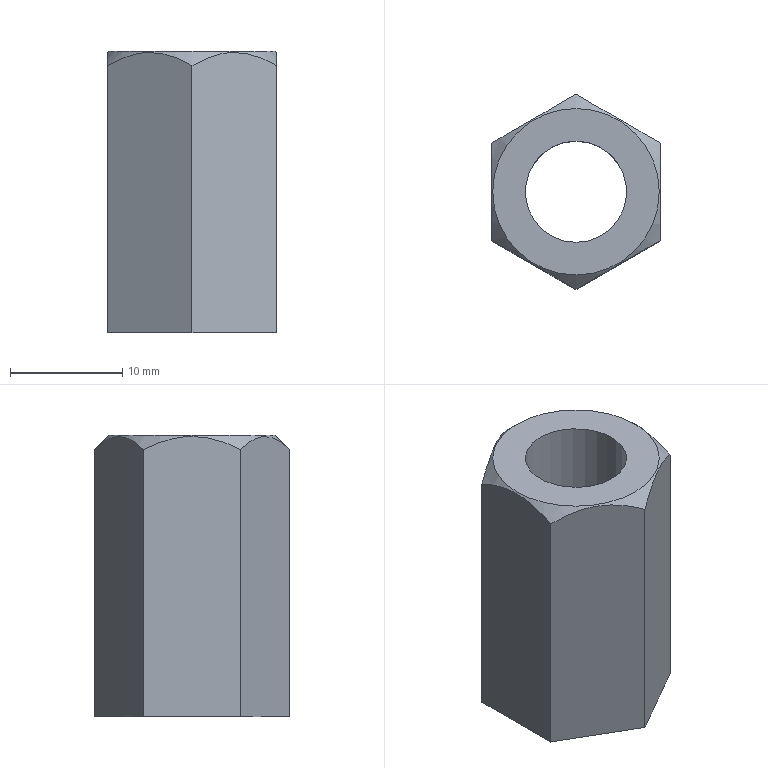Part | STEP file | 1 solid | 16 faces | box 15 x 17.321 x 25 mm | volume 2729 mm3 | plane 10 | cone 3 | cylinder 3 | commonest cylinder face diameters 9 x1 10.917 x1 12.5 x1
STEP:
#1=CARTESIAN_POINT('',(0.,0.,0.));
#2=DIRECTION('',(0.,0.,1.));
#3=DIRECTION('',(1.,0.,0.));
#4=AXIS2_PLACEMENT_3D('',#1,#2,#3);
#5=CARTESIAN_POINT('',(0.,-7.4,25.));
#6=VERTEX_POINT('',#5);
#7=CARTESIAN_POINT('',(0.,0.,25.));
#8=DIRECTION('',(0.,0.,-1.));
#9=DIRECTION('',(1.,0.,0.));
#10=AXIS2_PLACEMENT_3D('',#7,#8,#9);
#11=CIRCLE('',#10,7.4);
#12=CARTESIAN_POINT('',(0.,0.,23.4));
#13=DIRECTION('',(0.,0.,-1.));
#14=DIRECTION('',(0.,-1.,0.));
#15=AXIS2_PLACEMENT_3D('',#12,#13,#14);
#16=CONICAL_SURFACE('',#15,9.,0.7854);
#17=CARTESIAN_POINT('',(-1.571,-1.6));
#18=DIRECTION('',(1.,0.));
#19=VECTOR('',#18,1.);
#20=LINE('',#17,#19);
#21=(GEOMETRIC_REPRESENTATION_CONTEXT(2)PARAMETRIC_REPRESENTATION_CONTEXT()REPRESENTATION_CONTEXT('',''));
#22=DEFINITIONAL_REPRESENTATION('',(#20),#21);
#23=PCURVE('',#16,#22);
#24=CARTESIAN_POINT('',(0.,3.7,25.));
#25=DIRECTION('',(0.,0.,-1.));
#26=DIRECTION('',(-1.,0.,0.));
#27=AXIS2_PLACEMENT_3D('',#24,#25,#26);
#28=PLANE('',#27);
#29=CARTESIAN_POINT('',(0.,-3.7));
#30=DIRECTION('',(-1.,0.));
#31=AXIS2_PLACEMENT_2D('',#29,#30);
#32=CIRCLE('',#31,7.4);
#33=(GEOMETRIC_REPRESENTATION_CONTEXT(2)PARAMETRIC_REPRESENTATION_CONTEXT()REPRESENTATION_CONTEXT('',''));
#34=DEFINITIONAL_REPRESENTATION('',(#32),#33);
#35=PCURVE('',#28,#34);
#36=SURFACE_CURVE('',#11,(#23,#35),.PCURVE_S1.);
#37=EDGE_CURVE('',#6,#6,#36,.T.);
#38=ORIENTED_EDGE('',*,*,#37,.T.);
#39=CARTESIAN_POINT('',(0.,-8.66,23.74));
#40=VERTEX_POINT('',#39);
#41=CARTESIAN_POINT('',(0.,-7.4,25.));
#42=CARTESIAN_POINT('',(0.,-8.66,23.74));
#43=B_SPLINE_CURVE_WITH_KNOTS('',1,(#41,#42),.UNSPECIFIED.,.F.,.F.,(2,2),(-2.263,-0.4805),.PIECEWISE_BEZIER_KNOTS.);
#44=CARTESIAN_POINT('',(6.283,0.));
#45=DIRECTION('',(0.,1.));
#46=VECTOR('',#45,1.);
#47=LINE('',#44,#46);
#48=(GEOMETRIC_REPRESENTATION_CONTEXT(2)PARAMETRIC_REPRESENTATION_CONTEXT()REPRESENTATION_CONTEXT('',''));
#49=DEFINITIONAL_REPRESENTATION('',(#47),#48);
#50=PCURVE('',#16,#49);
#51=CARTESIAN_POINT('',(0.,0.));
#52=DIRECTION('',(0.,1.));
#53=VECTOR('',#52,1.);
#54=LINE('',#51,#53);
#55=(GEOMETRIC_REPRESENTATION_CONTEXT(2)PARAMETRIC_REPRESENTATION_CONTEXT()REPRESENTATION_CONTEXT('',''));
#56=DEFINITIONAL_REPRESENTATION('',(#54),#55);
#57=PCURVE('',#16,#56);
#58=SEAM_CURVE('',#43,(#50,#57),.PCURVE_S1.);
#59=EDGE_CURVE('',#6,#40,#58,.T.);
#60=ORIENTED_EDGE('',*,*,#59,.T.);
#61=CARTESIAN_POINT('',(7.5,-4.33,23.74));
#62=VERTEX_POINT('',#61);
#63=CARTESIAN_POINT('',(31.937,9.778,-1.));
#64=CARTESIAN_POINT('',(3.75,-6.495,30.716));
#65=CARTESIAN_POINT('',(-24.437,-22.769,-1.));
#66=(BOUNDED_CURVE()B_SPLINE_CURVE(2,(#63,#64,#65),.UNSPECIFIED.,.F.,.F.)B_SPLINE_CURVE_WITH_KNOTS((3,3),(0.,8.319),.PIECEWISE_BEZIER_KNOTS.)CURVE()GEOMETRIC_REPRESENTATION_ITEM()RATIONAL_B_SPLINE_CURVE((1.,4.453,1.))REPRESENTATION_ITEM(''));
#67=CARTESIAN_POINT('',(5.236,-0.3397));
#68=CARTESIAN_POINT('',(5.251,-0.4155));
#69=CARTESIAN_POINT('',(5.282,-0.558));
#70=CARTESIAN_POINT('',(5.328,-0.7466));
#71=CARTESIAN_POINT('',(5.375,-0.9116));
#72=CARTESIAN_POINT('',(5.422,-1.054));
#73=CARTESIAN_POINT('',(5.469,-1.176));
#74=CARTESIAN_POINT('',(5.517,-1.277));
#75=CARTESIAN_POINT('',(5.565,-1.359));
#76=CARTESIAN_POINT('',(5.614,-1.423));
#77=CARTESIAN_POINT('',(5.662,-1.467));
#78=CARTESIAN_POINT('',(5.711,-1.494));
#79=CARTESIAN_POINT('',(5.76,-1.503));
#80=CARTESIAN_POINT('',(5.808,-1.494));
#81=CARTESIAN_POINT('',(5.857,-1.467));
#82=CARTESIAN_POINT('',(5.906,-1.423));
#83=CARTESIAN_POINT('',(5.954,-1.359));
#84=CARTESIAN_POINT('',(6.002,-1.277));
#85=CARTESIAN_POINT('',(6.05,-1.176));
#86=CARTESIAN_POINT('',(6.097,-1.054));
#87=CARTESIAN_POINT('',(6.145,-0.9116));
#88=CARTESIAN_POINT('',(6.191,-0.7466));
#89=CARTESIAN_POINT('',(6.238,-0.558));
#90=CARTESIAN_POINT('',(6.268,-0.4155));
#91=CARTESIAN_POINT('',(6.283,-0.3397));
#92=B_SPLINE_CURVE_WITH_KNOTS('',3,(#67,#68,#69,#70,#71,#72,#73,#74,#75,#76,#77,#78,#79,#80,#81,#82,#83,#84,#85,#86,#87,#88,#89,#90,#91),.UNSPECIFIED.,.F.,.F.,(4,1,1,1,1,1,1,1,1,1,1,1,1,1,1,1,1,1,1,1,1,1,4),(2.759,2.886,3.014,3.141,3.268,3.396,3.523,3.65,3.777,3.905,4.032,4.159,4.287,4.414,4.541,4.669,4.796,4.923,5.051,5.178,5.305,5.433,5.56),.QUASI_UNIFORM_KNOTS.);
#93=(GEOMETRIC_REPRESENTATION_CONTEXT(2)PARAMETRIC_REPRESENTATION_CONTEXT()REPRESENTATION_CONTEXT('',''));
#94=DEFINITIONAL_REPRESENTATION('',(#92),#93);
#95=PCURVE('',#16,#94);
#96=CARTESIAN_POINT('',(-7.5,-12.99,0.));
#97=DIRECTION('',(-0.5,0.866,0.));
#98=DIRECTION('',(0.,0.,1.));
#99=AXIS2_PLACEMENT_3D('',#96,#97,#98);
#100=PLANE('',#99);
#101=CARTESIAN_POINT('',(-1.,45.537));
#102=CARTESIAN_POINT('',(30.716,12.99));
#103=CARTESIAN_POINT('',(-1.,-19.557));
#104=(BOUNDED_CURVE()B_SPLINE_CURVE(2,(#101,#102,#103),.UNSPECIFIED.,.F.,.F.)B_SPLINE_CURVE_WITH_KNOTS((3,3),(0.,8.319),.PIECEWISE_BEZIER_KNOTS.)CURVE()GEOMETRIC_REPRESENTATION_ITEM()RATIONAL_B_SPLINE_CURVE((1.,4.453,1.))REPRESENTATION_ITEM(''));
#105=(GEOMETRIC_REPRESENTATION_CONTEXT(2)PARAMETRIC_REPRESENTATION_CONTEXT()REPRESENTATION_CONTEXT('',''));
#106=DEFINITIONAL_REPRESENTATION('',(#104),#105);
#107=PCURVE('',#100,#106);
#108=SURFACE_CURVE('',#66,(#95,#107),.PCURVE_S1.);
#109=EDGE_CURVE('',#62,#40,#108,.T.);
#110=ORIENTED_EDGE('',*,*,#109,.F.);
#111=CARTESIAN_POINT('',(7.5,4.33,23.74));
#112=VERTEX_POINT('',#111);
#113=CARTESIAN_POINT('',(7.5,32.547,-1.));
#114=CARTESIAN_POINT('',(7.5,0.,30.716));
#115=CARTESIAN_POINT('',(7.5,-32.547,-1.));
#116=(BOUNDED_CURVE()B_SPLINE_CURVE(2,(#113,#114,#115),.UNSPECIFIED.,.F.,.F.)B_SPLINE_CURVE_WITH_KNOTS((3,3),(0.,8.319),.PIECEWISE_BEZIER_KNOTS.)CURVE()GEOMETRIC_REPRESENTATION_ITEM()RATIONAL_B_SPLINE_CURVE((1.,4.453,1.))REPRESENTATION_ITEM(''));
#117=CARTESIAN_POINT('',(4.189,-0.3397));
#118=CARTESIAN_POINT('',(4.204,-0.4155));
#119=CARTESIAN_POINT('',(4.234,-0.558));
#120=CARTESIAN_POINT('',(4.281,-0.7466));
#121=CARTESIAN_POINT('',(4.327,-0.9116));
#122=CARTESIAN_POINT('',(4.375,-1.054));
#123=CARTESIAN_POINT('',(4.422,-1.176));
#124=CARTESIAN_POINT('',(4.47,-1.277));
#125=CARTESIAN_POINT('',(4.518,-1.359));
#126=CARTESIAN_POINT('',(4.566,-1.423));
#127=CARTESIAN_POINT('',(4.615,-1.467));
#128=CARTESIAN_POINT('',(4.664,-1.494));
#129=CARTESIAN_POINT('',(4.712,-1.503));
#130=CARTESIAN_POINT('',(4.761,-1.494));
#131=CARTESIAN_POINT('',(4.81,-1.467));
#132=CARTESIAN_POINT('',(4.858,-1.423));
#133=CARTESIAN_POINT('',(4.907,-1.359));
#134=CARTESIAN_POINT('',(4.955,-1.277));
#135=CARTESIAN_POINT('',(5.003,-1.176));
#136=CARTESIAN_POINT('',(5.05,-1.054));
#137=CARTESIAN_POINT('',(5.097,-0.9116));
#138=CARTESIAN_POINT('',(5.144,-0.7466));
#139=CARTESIAN_POINT('',(5.19,-0.558));
#140=CARTESIAN_POINT('',(5.221,-0.4155));
#141=CARTESIAN_POINT('',(5.236,-0.3397));
#142=B_SPLINE_CURVE_WITH_KNOTS('',3,(#117,#118,#119,#120,#121,#122,#123,#124,#125,#126,#127,#128,#129,#130,#131,#132,#133,#134,#135,#136,#137,#138,#139,#140,#141),.UNSPECIFIED.,.F.,.F.,(4,1,1,1,1,1,1,1,1,1,1,1,1,1,1,1,1,1,1,1,1,1,4),(2.759,2.886,3.014,3.141,3.268,3.396,3.523,3.65,3.777,3.905,4.032,4.159,4.287,4.414,4.541,4.669,4.796,4.923,5.051,5.178,5.305,5.433,5.56),.QUASI_UNIFORM_KNOTS.);
#143=(GEOMETRIC_REPRESENTATION_CONTEXT(2)PARAMETRIC_REPRESENTATION_CONTEXT()REPRESENTATION_CONTEXT('',''));
#144=DEFINITIONAL_REPRESENTATION('',(#142),#143);
#145=PCURVE('',#16,#144);
#146=CARTESIAN_POINT('',(7.5,-4.33,0.));
#147=DIRECTION('',(-1.,0.,0.));
#148=DIRECTION('',(0.,0.,1.));
#149=AXIS2_PLACEMENT_3D('',#146,#147,#148);
#150=PLANE('',#149);
#151=CARTESIAN_POINT('',(-1.,36.877));
#152=CARTESIAN_POINT('',(30.716,4.33));
#153=CARTESIAN_POINT('',(-1.,-28.217));
#154=(BOUNDED_CURVE()B_SPLINE_CURVE(2,(#151,#152,#153),.UNSPECIFIED.,.F.,.F.)B_SPLINE_CURVE_WITH_KNOTS((3,3),(0.,8.319),.PIECEWISE_BEZIER_KNOTS.)CURVE()GEOMETRIC_REPRESENTATION_ITEM()RATIONAL_B_SPLINE_CURVE((1.,4.453,1.))REPRESENTATION_ITEM(''));
#155=(GEOMETRIC_REPRESENTATION_CONTEXT(2)PARAMETRIC_REPRESENTATION_CONTEXT()REPRESENTATION_CONTEXT('',''));
#156=DEFINITIONAL_REPRESENTATION('',(#154),#155);
#157=PCURVE('',#150,#156);
#158=SURFACE_CURVE('',#116,(#145,#157),.PCURVE_S1.);
#159=EDGE_CURVE('',#112,#62,#158,.T.);
#160=ORIENTED_EDGE('',*,*,#159,.F.);
#161=CARTESIAN_POINT('',(0.,8.66,23.74));
#162=VERTEX_POINT('',#161);
#163=CARTESIAN_POINT('',(-24.437,22.769,-1.));
#164=CARTESIAN_POINT('',(3.75,6.495,30.716));
#165=CARTESIAN_POINT('',(31.937,-9.778,-1.));
#166=(BOUNDED_CURVE()B_SPLINE_CURVE(2,(#163,#164,#165),.UNSPECIFIED.,.F.,.F.)B_SPLINE_CURVE_WITH_KNOTS((3,3),(0.,8.319),.PIECEWISE_BEZIER_KNOTS.)CURVE()GEOMETRIC_REPRESENTATION_ITEM()RATIONAL_B_SPLINE_CURVE((1.,4.453,1.))REPRESENTATION_ITEM(''));
#167=CARTESIAN_POINT('',(3.142,-0.3397));
#168=CARTESIAN_POINT('',(3.157,-0.4155));
#169=CARTESIAN_POINT('',(3.187,-0.558));
#170=CARTESIAN_POINT('',(3.233,-0.7466));
#171=CARTESIAN_POINT('',(3.28,-0.9116));
#172=CARTESIAN_POINT('',(3.327,-1.054));
#173=CARTESIAN_POINT('',(3.375,-1.176));
#174=CARTESIAN_POINT('',(3.423,-1.277));
#175=CARTESIAN_POINT('',(3.471,-1.359));
#176=CARTESIAN_POINT('',(3.519,-1.423));
#177=CARTESIAN_POINT('',(3.568,-1.467));
#178=CARTESIAN_POINT('',(3.616,-1.494));
#179=CARTESIAN_POINT('',(3.665,-1.503));
#180=CARTESIAN_POINT('',(3.714,-1.494));
#181=CARTESIAN_POINT('',(3.763,-1.467));
#182=CARTESIAN_POINT('',(3.811,-1.423));
#183=CARTESIAN_POINT('',(3.859,-1.359));
#184=CARTESIAN_POINT('',(3.908,-1.277));
#185=CARTESIAN_POINT('',(3.956,-1.176));
#186=CARTESIAN_POINT('',(4.003,-1.054));
#187=CARTESIAN_POINT('',(4.05,-0.9116));
#188=CARTESIAN_POINT('',(4.097,-0.7466));
#189=CARTESIAN_POINT('',(4.143,-0.558));
#190=CARTESIAN_POINT('',(4.174,-0.4155));
#191=CARTESIAN_POINT('',(4.189,-0.3397));
#192=B_SPLINE_CURVE_WITH_KNOTS('',3,(#167,#168,#169,#170,#171,#172,#173,#174,#175,#176,#177,#178,#179,#180,#181,#182,#183,#184,#185,#186,#187,#188,#189,#190,#191),.UNSPECIFIED.,.F.,.F.,(4,1,1,1,1,1,1,1,1,1,1,1,1,1,1,1,1,1,1,1,1,1,4),(2.759,2.886,3.014,3.141,3.268,3.396,3.523,3.65,3.777,3.905,4.032,4.159,4.287,4.414,4.541,4.669,4.796,4.923,5.051,5.178,5.305,5.433,5.56),.QUASI_UNIFORM_KNOTS.);
#193=(GEOMETRIC_REPRESENTATION_CONTEXT(2)PARAMETRIC_REPRESENTATION_CONTEXT()REPRESENTATION_CONTEXT('',''));
#194=DEFINITIONAL_REPRESENTATION('',(#192),#193);
#195=PCURVE('',#16,#194);
#196=CARTESIAN_POINT('',(7.5,4.33,0.));
#197=DIRECTION('',(-0.5,-0.866,0.));
#198=DIRECTION('',(0.,0.,1.));
#199=AXIS2_PLACEMENT_3D('',#196,#197,#198);
#200=PLANE('',#199);
#201=CARTESIAN_POINT('',(-1.,36.877));
#202=CARTESIAN_POINT('',(30.716,4.33));
#203=CARTESIAN_POINT('',(-1.,-28.217));
#204=(BOUNDED_CURVE()B_SPLINE_CURVE(2,(#201,#202,#203),.UNSPECIFIED.,.F.,.F.)B_SPLINE_CURVE_WITH_KNOTS((3,3),(0.,8.319),.PIECEWISE_BEZIER_KNOTS.)CURVE()GEOMETRIC_REPRESENTATION_ITEM()RATIONAL_B_SPLINE_CURVE((1.,4.453,1.))REPRESENTATION_ITEM(''));
#205=(GEOMETRIC_REPRESENTATION_CONTEXT(2)PARAMETRIC_REPRESENTATION_CONTEXT()REPRESENTATION_CONTEXT('',''));
#206=DEFINITIONAL_REPRESENTATION('',(#204),#205);
#207=PCURVE('',#200,#206);
#208=SURFACE_CURVE('',#166,(#195,#207),.PCURVE_S1.);
#209=EDGE_CURVE('',#162,#112,#208,.T.);
#210=ORIENTED_EDGE('',*,*,#209,.F.);
#211=CARTESIAN_POINT('',(-7.5,4.33,23.74));
#212=VERTEX_POINT('',#211);
#213=CARTESIAN_POINT('',(-31.937,-9.778,-1.));
#214=CARTESIAN_POINT('',(-3.75,6.495,30.716));
#215=CARTESIAN_POINT('',(24.437,22.769,-1.));
#216=(BOUNDED_CURVE()B_SPLINE_CURVE(2,(#213,#214,#215),.UNSPECIFIED.,.F.,.F.)B_SPLINE_CURVE_WITH_KNOTS((3,3),(0.,8.319),.PIECEWISE_BEZIER_KNOTS.)CURVE()GEOMETRIC_REPRESENTATION_ITEM()RATIONAL_B_SPLINE_CURVE((1.,4.453,1.))REPRESENTATION_ITEM(''));
#217=CARTESIAN_POINT('',(2.094,-0.3397));
#218=CARTESIAN_POINT('',(2.11,-0.4155));
#219=CARTESIAN_POINT('',(2.14,-0.558));
#220=CARTESIAN_POINT('',(2.186,-0.7466));
#221=CARTESIAN_POINT('',(2.233,-0.9116));
#222=CARTESIAN_POINT('',(2.28,-1.054));
#223=CARTESIAN_POINT('',(2.328,-1.176));
#224=CARTESIAN_POINT('',(2.376,-1.277));
#225=CARTESIAN_POINT('',(2.424,-1.359));
#226=CARTESIAN_POINT('',(2.472,-1.423));
#227=CARTESIAN_POINT('',(2.521,-1.467));
#228=CARTESIAN_POINT('',(2.569,-1.494));
#229=CARTESIAN_POINT('',(2.618,-1.503));
#230=CARTESIAN_POINT('',(2.667,-1.494));
#231=CARTESIAN_POINT('',(2.715,-1.467));
#232=CARTESIAN_POINT('',(2.764,-1.423));
#233=CARTESIAN_POINT('',(2.812,-1.359));
#234=CARTESIAN_POINT('',(2.86,-1.277));
#235=CARTESIAN_POINT('',(2.908,-1.176));
#236=CARTESIAN_POINT('',(2.956,-1.054));
#237=CARTESIAN_POINT('',(3.003,-0.9116));
#238=CARTESIAN_POINT('',(3.05,-0.7466));
#239=CARTESIAN_POINT('',(3.096,-0.558));
#240=CARTESIAN_POINT('',(3.126,-0.4155));
#241=CARTESIAN_POINT('',(3.142,-0.3397));
#242=B_SPLINE_CURVE_WITH_KNOTS('',3,(#217,#218,#219,#220,#221,#222,#223,#224,#225,#226,#227,#228,#229,#230,#231,#232,#233,#234,#235,#236,#237,#238,#239,#240,#241),.UNSPECIFIED.,.F.,.F.,(4,1,1,1,1,1,1,1,1,1,1,1,1,1,1,1,1,1,1,1,1,1,4),(2.759,2.886,3.014,3.141,3.268,3.396,3.523,3.65,3.777,3.905,4.032,4.159,4.287,4.414,4.541,4.669,4.796,4.923,5.051,5.178,5.305,5.433,5.56),.QUASI_UNIFORM_KNOTS.);
#243=(GEOMETRIC_REPRESENTATION_CONTEXT(2)PARAMETRIC_REPRESENTATION_CONTEXT()REPRESENTATION_CONTEXT('',''));
#244=DEFINITIONAL_REPRESENTATION('',(#242),#243);
#245=PCURVE('',#16,#244);
#246=CARTESIAN_POINT('',(7.5,12.99,0.));
#247=DIRECTION('',(0.5,-0.866,0.));
#248=DIRECTION('',(0.,0.,-1.));
#249=AXIS2_PLACEMENT_3D('',#246,#247,#248);
#250=PLANE('',#249);
#251=CARTESIAN_POINT('',(1.,-45.537));
#252=CARTESIAN_POINT('',(-30.716,-12.99));
#253=CARTESIAN_POINT('',(1.,19.557));
#254=(BOUNDED_CURVE()B_SPLINE_CURVE(2,(#251,#252,#253),.UNSPECIFIED.,.F.,.F.)B_SPLINE_CURVE_WITH_KNOTS((3,3),(0.,8.319),.PIECEWISE_BEZIER_KNOTS.)CURVE()GEOMETRIC_REPRESENTATION_ITEM()RATIONAL_B_SPLINE_CURVE((1.,4.453,1.))REPRESENTATION_ITEM(''));
#255=(GEOMETRIC_REPRESENTATION_CONTEXT(2)PARAMETRIC_REPRESENTATION_CONTEXT()REPRESENTATION_CONTEXT('',''));
#256=DEFINITIONAL_REPRESENTATION('',(#254),#255);
#257=PCURVE('',#250,#256);
#258=SURFACE_CURVE('',#216,(#245,#257),.PCURVE_S1.);
#259=EDGE_CURVE('',#212,#162,#258,.T.);
#260=ORIENTED_EDGE('',*,*,#259,.F.);
#261=CARTESIAN_POINT('',(-7.5,-4.33,23.74));
#262=VERTEX_POINT('',#261);
#263=CARTESIAN_POINT('',(-7.5,-32.547,-1.));
#264=CARTESIAN_POINT('',(-7.5,0.,30.716));
#265=CARTESIAN_POINT('',(-7.5,32.547,-1.));
#266=(BOUNDED_CURVE()B_SPLINE_CURVE(2,(#263,#264,#265),.UNSPECIFIED.,.F.,.F.)B_SPLINE_CURVE_WITH_KNOTS((3,3),(0.,8.319),.PIECEWISE_BEZIER_KNOTS.)CURVE()GEOMETRIC_REPRESENTATION_ITEM()RATIONAL_B_SPLINE_CURVE((1.,4.453,1.))REPRESENTATION_ITEM(''));
#267=CARTESIAN_POINT('',(1.047,-0.3397));
#268=CARTESIAN_POINT('',(1.062,-0.4155));
#269=CARTESIAN_POINT('',(1.093,-0.558));
#270=CARTESIAN_POINT('',(1.139,-0.7466));
#271=CARTESIAN_POINT('',(1.186,-0.9116));
#272=CARTESIAN_POINT('',(1.233,-1.054));
#273=CARTESIAN_POINT('',(1.28,-1.176));
#274=CARTESIAN_POINT('',(1.328,-1.277));
#275=CARTESIAN_POINT('',(1.376,-1.359));
#276=CARTESIAN_POINT('',(1.425,-1.423));
#277=CARTESIAN_POINT('',(1.473,-1.467));
#278=CARTESIAN_POINT('',(1.522,-1.494));
#279=CARTESIAN_POINT('',(1.571,-1.503));
#280=CARTESIAN_POINT('',(1.62,-1.494));
#281=CARTESIAN_POINT('',(1.668,-1.467));
#282=CARTESIAN_POINT('',(1.717,-1.423));
#283=CARTESIAN_POINT('',(1.765,-1.359));
#284=CARTESIAN_POINT('',(1.813,-1.277));
#285=CARTESIAN_POINT('',(1.861,-1.176));
#286=CARTESIAN_POINT('',(1.909,-1.054));
#287=CARTESIAN_POINT('',(1.956,-0.9116));
#288=CARTESIAN_POINT('',(2.003,-0.7466));
#289=CARTESIAN_POINT('',(2.049,-0.558));
#290=CARTESIAN_POINT('',(2.079,-0.4155));
#291=CARTESIAN_POINT('',(2.094,-0.3397));
#292=B_SPLINE_CURVE_WITH_KNOTS('',3,(#267,#268,#269,#270,#271,#272,#273,#274,#275,#276,#277,#278,#279,#280,#281,#282,#283,#284,#285,#286,#287,#288,#289,#290,#291),.UNSPECIFIED.,.F.,.F.,(4,1,1,1,1,1,1,1,1,1,1,1,1,1,1,1,1,1,1,1,1,1,4),(2.759,2.886,3.014,3.141,3.268,3.396,3.523,3.65,3.777,3.905,4.032,4.159,4.287,4.414,4.541,4.669,4.796,4.923,5.051,5.178,5.305,5.433,5.56),.QUASI_UNIFORM_KNOTS.);
#293=(GEOMETRIC_REPRESENTATION_CONTEXT(2)PARAMETRIC_REPRESENTATION_CONTEXT()REPRESENTATION_CONTEXT('',''));
#294=DEFINITIONAL_REPRESENTATION('',(#292),#293);
#295=PCURVE('',#16,#294);
#296=CARTESIAN_POINT('',(-7.5,4.33,0.));
#297=DIRECTION('',(1.,0.,0.));
#298=DIRECTION('',(0.,0.,-1.));
#299=AXIS2_PLACEMENT_3D('',#296,#297,#298);
#300=PLANE('',#299);
#301=CARTESIAN_POINT('',(1.,-36.877));
#302=CARTESIAN_POINT('',(-30.716,-4.33));
#303=CARTESIAN_POINT('',(1.,28.217));
#304=(BOUNDED_CURVE()B_SPLINE_CURVE(2,(#301,#302,#303),.UNSPECIFIED.,.F.,.F.)B_SPLINE_CURVE_WITH_KNOTS((3,3),(0.,8.319),.PIECEWISE_BEZIER_KNOTS.)CURVE()GEOMETRIC_REPRESENTATION_ITEM()RATIONAL_B_SPLINE_CURVE((1.,4.453,1.))REPRESENTATION_ITEM(''));
#305=(GEOMETRIC_REPRESENTATION_CONTEXT(2)PARAMETRIC_REPRESENTATION_CONTEXT()REPRESENTATION_CONTEXT('',''));
#306=DEFINITIONAL_REPRESENTATION('',(#304),#305);
#307=PCURVE('',#300,#306);
#308=SURFACE_CURVE('',#266,(#295,#307),.PCURVE_S1.);
#309=EDGE_CURVE('',#262,#212,#308,.T.);
#310=ORIENTED_EDGE('',*,*,#309,.F.);
#311=CARTESIAN_POINT('',(24.437,-22.769,-1.));
#312=CARTESIAN_POINT('',(-3.75,-6.495,30.716));
#313=CARTESIAN_POINT('',(-31.937,9.778,-1.));
#314=(BOUNDED_CURVE()B_SPLINE_CURVE(2,(#311,#312,#313),.UNSPECIFIED.,.F.,.F.)B_SPLINE_CURVE_WITH_KNOTS((3,3),(0.,8.319),.PIECEWISE_BEZIER_KNOTS.)CURVE()GEOMETRIC_REPRESENTATION_ITEM()RATIONAL_B_SPLINE_CURVE((1.,4.453,1.))REPRESENTATION_ITEM(''));
#315=CARTESIAN_POINT('',(0.,-0.3397));
#316=CARTESIAN_POINT('',(0.01515,-0.4155));
#317=CARTESIAN_POINT('',(0.04564,-0.558));
#318=CARTESIAN_POINT('',(0.09189,-0.7466));
#319=CARTESIAN_POINT('',(0.1386,-0.9116));
#320=CARTESIAN_POINT('',(0.1858,-1.054));
#321=CARTESIAN_POINT('',(0.2333,-1.176));
#322=CARTESIAN_POINT('',(0.2812,-1.277));
#323=CARTESIAN_POINT('',(0.3293,-1.359));
#324=CARTESIAN_POINT('',(0.3777,-1.423));
#325=CARTESIAN_POINT('',(0.4262,-1.467));
#326=CARTESIAN_POINT('',(0.4749,-1.494));
#327=CARTESIAN_POINT('',(0.5236,-1.503));
#328=CARTESIAN_POINT('',(0.5723,-1.494));
#329=CARTESIAN_POINT('',(0.621,-1.467));
#330=CARTESIAN_POINT('',(0.6695,-1.423));
#331=CARTESIAN_POINT('',(0.7179,-1.359));
#332=CARTESIAN_POINT('',(0.766,-1.277));
#333=CARTESIAN_POINT('',(0.8139,-1.176));
#334=CARTESIAN_POINT('',(0.8614,-1.054));
#335=CARTESIAN_POINT('',(0.9086,-0.9116));
#336=CARTESIAN_POINT('',(0.9553,-0.7466));
#337=CARTESIAN_POINT('',(1.002,-0.558));
#338=CARTESIAN_POINT('',(1.032,-0.4155));
#339=CARTESIAN_POINT('',(1.047,-0.3397));
#340=B_SPLINE_CURVE_WITH_KNOTS('',3,(#315,#316,#317,#318,#319,#320,#321,#322,#323,#324,#325,#326,#327,#328,#329,#330,#331,#332,#333,#334,#335,#336,#337,#338,#339),.UNSPECIFIED.,.F.,.F.,(4,1,1,1,1,1,1,1,1,1,1,1,1,1,1,1,1,1,1,1,1,1,4),(2.759,2.886,3.014,3.141,3.268,3.396,3.523,3.65,3.777,3.905,4.032,4.159,4.287,4.414,4.541,4.669,4.796,4.923,5.051,5.178,5.305,5.433,5.56),.QUASI_UNIFORM_KNOTS.);
#341=(GEOMETRIC_REPRESENTATION_CONTEXT(2)PARAMETRIC_REPRESENTATION_CONTEXT()REPRESENTATION_CONTEXT('',''));
#342=DEFINITIONAL_REPRESENTATION('',(#340),#341);
#343=PCURVE('',#16,#342);
#344=CARTESIAN_POINT('',(-7.5,-4.33,0.));
#345=DIRECTION('',(0.5,0.866,0.));
#346=DIRECTION('',(0.,0.,-1.));
#347=AXIS2_PLACEMENT_3D('',#344,#345,#346);
#348=PLANE('',#347);
#349=CARTESIAN_POINT('',(1.,-36.877));
#350=CARTESIAN_POINT('',(-30.716,-4.33));
#351=CARTESIAN_POINT('',(1.,28.217));
#352=(BOUNDED_CURVE()B_SPLINE_CURVE(2,(#349,#350,#351),.UNSPECIFIED.,.F.,.F.)B_SPLINE_CURVE_WITH_KNOTS((3,3),(0.,8.319),.PIECEWISE_BEZIER_KNOTS.)CURVE()GEOMETRIC_REPRESENTATION_ITEM()RATIONAL_B_SPLINE_CURVE((1.,4.453,1.))REPRESENTATION_ITEM(''));
#353=(GEOMETRIC_REPRESENTATION_CONTEXT(2)PARAMETRIC_REPRESENTATION_CONTEXT()REPRESENTATION_CONTEXT('',''));
#354=DEFINITIONAL_REPRESENTATION('',(#352),#353);
#355=PCURVE('',#348,#354);
#356=SURFACE_CURVE('',#314,(#343,#355),.PCURVE_S1.);
#357=EDGE_CURVE('',#40,#262,#356,.T.);
#358=ORIENTED_EDGE('',*,*,#357,.F.);
#359=ORIENTED_EDGE('',*,*,#59,.F.);
#360=EDGE_LOOP('',(#38,#60,#110,#160,#210,#260,#310,#358,#359));
#361=FACE_BOUND('',#360,.T.);
#362=ADVANCED_FACE('',(#361),#16,.T.);
#363=ORIENTED_EDGE('',*,*,#37,.F.);
#364=EDGE_LOOP('',(#363));
#365=FACE_BOUND('',#364,.T.);
#366=CARTESIAN_POINT('',(0.,-4.5,25.));
#367=VERTEX_POINT('',#366);
#368=CARTESIAN_POINT('',(0.,0.,25.));
#369=DIRECTION('',(0.,0.,1.));
#370=DIRECTION('',(0.,1.,0.));
#371=AXIS2_PLACEMENT_3D('',#368,#369,#370);
#372=CIRCLE('',#371,4.5);
#373=CARTESIAN_POINT('',(0.,0.8));
#374=CARTESIAN_POINT('',(7.794,0.8));
#375=CARTESIAN_POINT('',(3.897,-5.95));
#376=CARTESIAN_POINT('',(0.,-12.7));
#377=CARTESIAN_POINT('',(-3.897,-5.95));
#378=CARTESIAN_POINT('',(-7.794,0.8));
#379=CARTESIAN_POINT('',(0.,0.8));
#380=(BOUNDED_CURVE()B_SPLINE_CURVE(2,(#373,#374,#375,#376,#377,#378,#379),.UNSPECIFIED.,.T.,.F.)B_SPLINE_CURVE_WITH_KNOTS((1,2,2,2,2,1),(-2.094,0.,2.094,4.189,6.283,8.378),.UNSPECIFIED.)CURVE()GEOMETRIC_REPRESENTATION_ITEM()RATIONAL_B_SPLINE_CURVE((1.,0.5,1.,0.5,1.,0.5,1.))REPRESENTATION_ITEM(''));
#381=(GEOMETRIC_REPRESENTATION_CONTEXT(2)PARAMETRIC_REPRESENTATION_CONTEXT()REPRESENTATION_CONTEXT('',''));
#382=DEFINITIONAL_REPRESENTATION('',(#380),#381);
#383=PCURVE('',#28,#382);
#384=CARTESIAN_POINT('',(0.,0.,20.25));
#385=DIRECTION('',(0.,0.,1.));
#386=DIRECTION('',(0.,-1.,0.));
#387=AXIS2_PLACEMENT_3D('',#384,#385,#386);
#388=CYLINDRICAL_SURFACE('',#387,4.5);
#389=CARTESIAN_POINT('',(-3.142,4.75));
#390=DIRECTION('',(1.,0.));
#391=VECTOR('',#390,1.);
#392=LINE('',#389,#391);
#393=(GEOMETRIC_REPRESENTATION_CONTEXT(2)PARAMETRIC_REPRESENTATION_CONTEXT()REPRESENTATION_CONTEXT('',''));
#394=DEFINITIONAL_REPRESENTATION('',(#392),#393);
#395=PCURVE('',#388,#394);
#396=SURFACE_CURVE('',#372,(#383,#395),.PCURVE_S1.);
#397=EDGE_CURVE('',#367,#367,#396,.T.);
#398=ORIENTED_EDGE('',*,*,#397,.F.);
#399=EDGE_LOOP('',(#398));
#400=FACE_BOUND('',#399,.T.);
#401=ADVANCED_FACE('',(#365,#400),#28,.F.);
#402=CARTESIAN_POINT('',(0.,8.66,0.));
#403=VERTEX_POINT('',#402);
#404=CARTESIAN_POINT('',(0.000000001,8.66,23.74));
#405=DIRECTION('',(0.,0.,-1.));
#406=VECTOR('',#405,1.);
#407=LINE('',#404,#406);
#408=CARTESIAN_POINT('',(-23.74,-8.66));
#409=DIRECTION('',(1.,0.));
#410=VECTOR('',#409,1.);
#411=LINE('',#408,#410);
#412=(GEOMETRIC_REPRESENTATION_CONTEXT(2)PARAMETRIC_REPRESENTATION_CONTEXT()REPRESENTATION_CONTEXT('',''));
#413=DEFINITIONAL_REPRESENTATION('',(#411),#412);
#414=PCURVE('',#250,#413);
#415=CARTESIAN_POINT('',(23.74,8.66));
#416=DIRECTION('',(-1.,0.));
#417=VECTOR('',#416,1.);
#418=LINE('',#415,#417);
#419=(GEOMETRIC_REPRESENTATION_CONTEXT(2)PARAMETRIC_REPRESENTATION_CONTEXT()REPRESENTATION_CONTEXT('',''));
#420=DEFINITIONAL_REPRESENTATION('',(#418),#419);
#421=PCURVE('',#200,#420);
#422=SURFACE_CURVE('',#407,(#414,#421),.PCURVE_S1.);
#423=EDGE_CURVE('',#162,#403,#422,.T.);
#424=ORIENTED_EDGE('',*,*,#423,.T.);
#425=CARTESIAN_POINT('',(-7.5,4.33,0.));
#426=VERTEX_POINT('',#425);
#427=CARTESIAN_POINT('',(0.,8.66,0.));
#428=DIRECTION('',(-0.866,-0.5,0.));
#429=VECTOR('',#428,1.);
#430=LINE('',#427,#429);
#431=CARTESIAN_POINT('',(0.,-8.66));
#432=DIRECTION('',(0.,-1.));
#433=VECTOR('',#432,1.);
#434=LINE('',#431,#433);
#435=(GEOMETRIC_REPRESENTATION_CONTEXT(2)PARAMETRIC_REPRESENTATION_CONTEXT()REPRESENTATION_CONTEXT('',''));
#436=DEFINITIONAL_REPRESENTATION('',(#434),#435);
#437=PCURVE('',#250,#436);
#438=CARTESIAN_POINT('',(0.,4.5,0.));
#439=DIRECTION('',(0.,0.,-1.));
#440=DIRECTION('',(-1.,0.,0.));
#441=AXIS2_PLACEMENT_3D('',#438,#439,#440);
#442=PLANE('',#441);
#443=CARTESIAN_POINT('',(0.,4.16));
#444=DIRECTION('',(0.866,-0.5));
#445=VECTOR('',#444,1.);
#446=LINE('',#443,#445);
#447=(GEOMETRIC_REPRESENTATION_CONTEXT(2)PARAMETRIC_REPRESENTATION_CONTEXT()REPRESENTATION_CONTEXT('',''));
#448=DEFINITIONAL_REPRESENTATION('',(#446),#447);
#449=PCURVE('',#442,#448);
#450=SURFACE_CURVE('',#430,(#437,#449),.PCURVE_S1.);
#451=EDGE_CURVE('',#403,#426,#450,.T.);
#452=ORIENTED_EDGE('',*,*,#451,.T.);
#453=CARTESIAN_POINT('',(-7.5,4.33,0.));
#454=DIRECTION('',(0.,0.,1.));
#455=VECTOR('',#454,1.);
#456=LINE('',#453,#455);
#457=CARTESIAN_POINT('',(0.,-17.321));
#458=DIRECTION('',(-1.,0.));
#459=VECTOR('',#458,1.);
#460=LINE('',#457,#459);
#461=(GEOMETRIC_REPRESENTATION_CONTEXT(2)PARAMETRIC_REPRESENTATION_CONTEXT()REPRESENTATION_CONTEXT('',''));
#462=DEFINITIONAL_REPRESENTATION('',(#460),#461);
#463=PCURVE('',#250,#462);
#464=CARTESIAN_POINT('',(0.,0.));
#465=DIRECTION('',(-1.,0.));
#466=VECTOR('',#465,1.);
#467=LINE('',#464,#466);
#468=(GEOMETRIC_REPRESENTATION_CONTEXT(2)PARAMETRIC_REPRESENTATION_CONTEXT()REPRESENTATION_CONTEXT('',''));
#469=DEFINITIONAL_REPRESENTATION('',(#467),#468);
#470=PCURVE('',#300,#469);
#471=SURFACE_CURVE('',#456,(#463,#470),.PCURVE_S1.);
#472=EDGE_CURVE('',#426,#212,#471,.T.);
#473=ORIENTED_EDGE('',*,*,#472,.T.);
#474=ORIENTED_EDGE('',*,*,#259,.T.);
#475=EDGE_LOOP('',(#424,#452,#473,#474));
#476=FACE_BOUND('',#475,.T.);
#477=ADVANCED_FACE('',(#476),#250,.F.);
#478=ORIENTED_EDGE('',*,*,#309,.T.);
#479=ORIENTED_EDGE('',*,*,#472,.F.);
#480=CARTESIAN_POINT('',(-7.5,-4.33,0.));
#481=VERTEX_POINT('',#480);
#482=CARTESIAN_POINT('',(-7.5,4.33,0.));
#483=DIRECTION('',(0.,-1.,0.));
#484=VECTOR('',#483,1.);
#485=LINE('',#482,#484);
#486=CARTESIAN_POINT('',(0.,0.000000001));
#487=DIRECTION('',(0.,-1.));
#488=VECTOR('',#487,1.);
#489=LINE('',#486,#488);
#490=(GEOMETRIC_REPRESENTATION_CONTEXT(2)PARAMETRIC_REPRESENTATION_CONTEXT()REPRESENTATION_CONTEXT('',''));
#491=DEFINITIONAL_REPRESENTATION('',(#489),#490);
#492=PCURVE('',#300,#491);
#493=CARTESIAN_POINT('',(7.5,-0.1699));
#494=DIRECTION('',(0.,-1.));
#495=VECTOR('',#494,1.);
#496=LINE('',#493,#495);
#497=(GEOMETRIC_REPRESENTATION_CONTEXT(2)PARAMETRIC_REPRESENTATION_CONTEXT()REPRESENTATION_CONTEXT('',''));
#498=DEFINITIONAL_REPRESENTATION('',(#496),#497);
#499=PCURVE('',#442,#498);
#500=SURFACE_CURVE('',#485,(#492,#499),.PCURVE_S1.);
#501=EDGE_CURVE('',#426,#481,#500,.T.);
#502=ORIENTED_EDGE('',*,*,#501,.T.);
#503=CARTESIAN_POINT('',(-7.5,-4.33,0.));
#504=DIRECTION('',(0.,0.,1.));
#505=VECTOR('',#504,1.);
#506=LINE('',#503,#505);
#507=CARTESIAN_POINT('',(0.,-8.66));
#508=DIRECTION('',(-1.,0.));
#509=VECTOR('',#508,1.);
#510=LINE('',#507,#509);
#511=(GEOMETRIC_REPRESENTATION_CONTEXT(2)PARAMETRIC_REPRESENTATION_CONTEXT()REPRESENTATION_CONTEXT('',''));
#512=DEFINITIONAL_REPRESENTATION('',(#510),#511);
#513=PCURVE('',#300,#512);
#514=CARTESIAN_POINT('',(0.,0.));
#515=DIRECTION('',(-1.,0.));
#516=VECTOR('',#515,1.);
#517=LINE('',#514,#516);
#518=(GEOMETRIC_REPRESENTATION_CONTEXT(2)PARAMETRIC_REPRESENTATION_CONTEXT()REPRESENTATION_CONTEXT('',''));
#519=DEFINITIONAL_REPRESENTATION('',(#517),#518);
#520=PCURVE('',#348,#519);
#521=SURFACE_CURVE('',#506,(#513,#520),.PCURVE_S1.);
#522=EDGE_CURVE('',#481,#262,#521,.T.);
#523=ORIENTED_EDGE('',*,*,#522,.T.);
#524=EDGE_LOOP('',(#478,#479,#502,#523));
#525=FACE_BOUND('',#524,.T.);
#526=ADVANCED_FACE('',(#525),#300,.F.);
#527=ORIENTED_EDGE('',*,*,#357,.T.);
#528=ORIENTED_EDGE('',*,*,#522,.F.);
#529=CARTESIAN_POINT('',(0.,-8.66,0.));
#530=VERTEX_POINT('',#529);
#531=CARTESIAN_POINT('',(-7.5,-4.33,0.));
#532=DIRECTION('',(0.866,-0.5,0.));
#533=VECTOR('',#532,1.);
#534=LINE('',#531,#533);
#535=CARTESIAN_POINT('',(0.,0.));
#536=DIRECTION('',(0.,-1.));
#537=VECTOR('',#536,1.);
#538=LINE('',#535,#537);
#539=(GEOMETRIC_REPRESENTATION_CONTEXT(2)PARAMETRIC_REPRESENTATION_CONTEXT()REPRESENTATION_CONTEXT('',''));
#540=DEFINITIONAL_REPRESENTATION('',(#538),#539);
#541=PCURVE('',#348,#540);
#542=CARTESIAN_POINT('',(7.5,-8.83));
#543=DIRECTION('',(-0.866,-0.5));
#544=VECTOR('',#543,1.);
#545=LINE('',#542,#544);
#546=(GEOMETRIC_REPRESENTATION_CONTEXT(2)PARAMETRIC_REPRESENTATION_CONTEXT()REPRESENTATION_CONTEXT('',''));
#547=DEFINITIONAL_REPRESENTATION('',(#545),#546);
#548=PCURVE('',#442,#547);
#549=SURFACE_CURVE('',#534,(#541,#548),.PCURVE_S1.);
#550=EDGE_CURVE('',#481,#530,#549,.T.);
#551=ORIENTED_EDGE('',*,*,#550,.T.);
#552=CARTESIAN_POINT('',(-0.000000001,-8.66,0.));
#553=DIRECTION('',(0.,0.,1.));
#554=VECTOR('',#553,1.);
#555=LINE('',#552,#554);
#556=CARTESIAN_POINT('',(0.,-8.66));
#557=DIRECTION('',(-1.,0.));
#558=VECTOR('',#557,1.);
#559=LINE('',#556,#558);
#560=(GEOMETRIC_REPRESENTATION_CONTEXT(2)PARAMETRIC_REPRESENTATION_CONTEXT()REPRESENTATION_CONTEXT('',''));
#561=DEFINITIONAL_REPRESENTATION('',(#559),#560);
#562=PCURVE('',#348,#561);
#563=CARTESIAN_POINT('',(0.,8.66));
#564=DIRECTION('',(1.,0.));
#565=VECTOR('',#564,1.);
#566=LINE('',#563,#565);
#567=(GEOMETRIC_REPRESENTATION_CONTEXT(2)PARAMETRIC_REPRESENTATION_CONTEXT()REPRESENTATION_CONTEXT('',''));
#568=DEFINITIONAL_REPRESENTATION('',(#566),#567);
#569=PCURVE('',#100,#568);
#570=SURFACE_CURVE('',#555,(#562,#569),.PCURVE_S1.);
#571=EDGE_CURVE('',#530,#40,#570,.T.);
#572=ORIENTED_EDGE('',*,*,#571,.T.);
#573=EDGE_LOOP('',(#527,#528,#551,#572));
#574=FACE_BOUND('',#573,.T.);
#575=ADVANCED_FACE('',(#574),#348,.F.);
#576=ORIENTED_EDGE('',*,*,#397,.F.);
#577=CARTESIAN_POINT('',(0.,-4.5,15.5));
#578=VERTEX_POINT('',#577);
#579=CARTESIAN_POINT('',(0.,-4.5,15.5));
#580=CARTESIAN_POINT('',(0.,-4.5,25.));
#581=B_SPLINE_CURVE_WITH_KNOTS('',1,(#579,#580),.UNSPECIFIED.,.F.,.F.,(2,2),(-4.75,4.75),.PIECEWISE_BEZIER_KNOTS.);
#582=CARTESIAN_POINT('',(0.,0.));
#583=DIRECTION('',(0.,1.));
#584=VECTOR('',#583,1.);
#585=LINE('',#582,#584);
#586=(GEOMETRIC_REPRESENTATION_CONTEXT(2)PARAMETRIC_REPRESENTATION_CONTEXT()REPRESENTATION_CONTEXT('',''));
#587=DEFINITIONAL_REPRESENTATION('',(#585),#586);
#588=PCURVE('',#388,#587);
#589=CARTESIAN_POINT('',(6.283,0.));
#590=DIRECTION('',(0.,1.));
#591=VECTOR('',#590,1.);
#592=LINE('',#589,#591);
#593=(GEOMETRIC_REPRESENTATION_CONTEXT(2)PARAMETRIC_REPRESENTATION_CONTEXT()REPRESENTATION_CONTEXT('',''));
#594=DEFINITIONAL_REPRESENTATION('',(#592),#593);
#595=PCURVE('',#388,#594);
#596=SEAM_CURVE('',#581,(#588,#595),.PCURVE_S1.);
#597=EDGE_CURVE('',#578,#367,#596,.T.);
#598=ORIENTED_EDGE('',*,*,#597,.F.);
#599=CARTESIAN_POINT('',(0.,0.,15.5));
#600=DIRECTION('',(0.,0.,1.));
#601=DIRECTION('',(1.,0.,0.));
#602=AXIS2_PLACEMENT_3D('',#599,#600,#601);
#603=CIRCLE('',#602,4.5);
#604=CARTESIAN_POINT('',(-4.712,-4.75));
#605=DIRECTION('',(1.,0.));
#606=VECTOR('',#605,1.);
#607=LINE('',#604,#606);
#608=(GEOMETRIC_REPRESENTATION_CONTEXT(2)PARAMETRIC_REPRESENTATION_CONTEXT()REPRESENTATION_CONTEXT('',''));
#609=DEFINITIONAL_REPRESENTATION('',(#607),#608);
#610=PCURVE('',#388,#609);
#611=CARTESIAN_POINT('',(0.,5.375,15.5));
#612=DIRECTION('',(0.,0.,-1.));
#613=DIRECTION('',(-1.,0.,0.));
#614=AXIS2_PLACEMENT_3D('',#611,#612,#613);
#615=PLANE('',#614);
#616=CARTESIAN_POINT('',(-4.5,-5.375));
#617=CARTESIAN_POINT('',(-4.5,2.419));
#618=CARTESIAN_POINT('',(2.25,-1.478));
#619=CARTESIAN_POINT('',(9.,-5.375));
#620=CARTESIAN_POINT('',(2.25,-9.272));
#621=CARTESIAN_POINT('',(-4.5,-13.169));
#622=CARTESIAN_POINT('',(-4.5,-5.375));
#623=(BOUNDED_CURVE()B_SPLINE_CURVE(2,(#616,#617,#618,#619,#620,#621,#622),.UNSPECIFIED.,.T.,.F.)B_SPLINE_CURVE_WITH_KNOTS((1,2,2,2,2,1),(-2.094,0.,2.094,4.189,6.283,8.378),.UNSPECIFIED.)CURVE()GEOMETRIC_REPRESENTATION_ITEM()RATIONAL_B_SPLINE_CURVE((1.,0.5,1.,0.5,1.,0.5,1.))REPRESENTATION_ITEM(''));
#624=(GEOMETRIC_REPRESENTATION_CONTEXT(2)PARAMETRIC_REPRESENTATION_CONTEXT()REPRESENTATION_CONTEXT('',''));
#625=DEFINITIONAL_REPRESENTATION('',(#623),#624);
#626=PCURVE('',#615,#625);
#627=SURFACE_CURVE('',#603,(#610,#626),.PCURVE_S1.);
#628=EDGE_CURVE('',#578,#578,#627,.T.);
#629=ORIENTED_EDGE('',*,*,#628,.T.);
#630=ORIENTED_EDGE('',*,*,#597,.T.);
#631=EDGE_LOOP('',(#576,#598,#629,#630));
#632=FACE_BOUND('',#631,.F.);
#633=ADVANCED_FACE('',(#632),#388,.F.);
#634=ORIENTED_EDGE('',*,*,#109,.T.);
#635=ORIENTED_EDGE('',*,*,#571,.F.);
#636=CARTESIAN_POINT('',(7.5,-4.33,0.));
#637=VERTEX_POINT('',#636);
#638=CARTESIAN_POINT('',(0.,-8.66,0.));
#639=DIRECTION('',(0.866,0.5,0.));
#640=VECTOR('',#639,1.);
#641=LINE('',#638,#640);
#642=CARTESIAN_POINT('',(0.,8.66));
#643=DIRECTION('',(0.,1.));
#644=VECTOR('',#643,1.);
#645=LINE('',#642,#644);
#646=(GEOMETRIC_REPRESENTATION_CONTEXT(2)PARAMETRIC_REPRESENTATION_CONTEXT()REPRESENTATION_CONTEXT('',''));
#647=DEFINITIONAL_REPRESENTATION('',(#645),#646);
#648=PCURVE('',#100,#647);
#649=CARTESIAN_POINT('',(0.,-13.16));
#650=DIRECTION('',(-0.866,0.5));
#651=VECTOR('',#650,1.);
#652=LINE('',#649,#651);
#653=(GEOMETRIC_REPRESENTATION_CONTEXT(2)PARAMETRIC_REPRESENTATION_CONTEXT()REPRESENTATION_CONTEXT('',''));
#654=DEFINITIONAL_REPRESENTATION('',(#652),#653);
#655=PCURVE('',#442,#654);
#656=SURFACE_CURVE('',#641,(#648,#655),.PCURVE_S1.);
#657=EDGE_CURVE('',#530,#637,#656,.T.);
#658=ORIENTED_EDGE('',*,*,#657,.T.);
#659=CARTESIAN_POINT('',(7.5,-4.33,0.));
#660=DIRECTION('',(0.,0.,1.));
#661=VECTOR('',#660,1.);
#662=LINE('',#659,#661);
#663=CARTESIAN_POINT('',(0.,17.321));
#664=DIRECTION('',(1.,0.));
#665=VECTOR('',#664,1.);
#666=LINE('',#663,#665);
#667=(GEOMETRIC_REPRESENTATION_CONTEXT(2)PARAMETRIC_REPRESENTATION_CONTEXT()REPRESENTATION_CONTEXT('',''));
#668=DEFINITIONAL_REPRESENTATION('',(#666),#667);
#669=PCURVE('',#100,#668);
#670=CARTESIAN_POINT('',(0.,0.));
#671=DIRECTION('',(1.,0.));
#672=VECTOR('',#671,1.);
#673=LINE('',#670,#672);
#674=(GEOMETRIC_REPRESENTATION_CONTEXT(2)PARAMETRIC_REPRESENTATION_CONTEXT()REPRESENTATION_CONTEXT('',''));
#675=DEFINITIONAL_REPRESENTATION('',(#673),#674);
#676=PCURVE('',#150,#675);
#677=SURFACE_CURVE('',#662,(#669,#676),.PCURVE_S1.);
#678=EDGE_CURVE('',#637,#62,#677,.T.);
#679=ORIENTED_EDGE('',*,*,#678,.T.);
#680=EDGE_LOOP('',(#634,#635,#658,#679));
#681=FACE_BOUND('',#680,.T.);
#682=ADVANCED_FACE('',(#681),#100,.F.);
#683=ORIENTED_EDGE('',*,*,#159,.T.);
#684=ORIENTED_EDGE('',*,*,#678,.F.);
#685=CARTESIAN_POINT('',(7.5,4.33,0.));
#686=VERTEX_POINT('',#685);
#687=CARTESIAN_POINT('',(7.5,-4.33,0.));
#688=DIRECTION('',(0.,1.,0.));
#689=VECTOR('',#688,1.);
#690=LINE('',#687,#689);
#691=CARTESIAN_POINT('',(0.,-0.000000001));
#692=DIRECTION('',(0.,1.));
#693=VECTOR('',#692,1.);
#694=LINE('',#691,#693);
#695=(GEOMETRIC_REPRESENTATION_CONTEXT(2)PARAMETRIC_REPRESENTATION_CONTEXT()REPRESENTATION_CONTEXT('',''));
#696=DEFINITIONAL_REPRESENTATION('',(#694),#695);
#697=PCURVE('',#150,#696);
#698=CARTESIAN_POINT('',(-7.5,-8.83));
#699=DIRECTION('',(0.,1.));
#700=VECTOR('',#699,1.);
#701=LINE('',#698,#700);
#702=(GEOMETRIC_REPRESENTATION_CONTEXT(2)PARAMETRIC_REPRESENTATION_CONTEXT()REPRESENTATION_CONTEXT('',''));
#703=DEFINITIONAL_REPRESENTATION('',(#701),#702);
#704=PCURVE('',#442,#703);
#705=SURFACE_CURVE('',#690,(#697,#704),.PCURVE_S1.);
#706=EDGE_CURVE('',#637,#686,#705,.T.);
#707=ORIENTED_EDGE('',*,*,#706,.T.);
#708=CARTESIAN_POINT('',(7.5,4.33,0.));
#709=DIRECTION('',(0.,0.,1.));
#710=VECTOR('',#709,1.);
#711=LINE('',#708,#710);
#712=CARTESIAN_POINT('',(0.,8.66));
#713=DIRECTION('',(1.,0.));
#714=VECTOR('',#713,1.);
#715=LINE('',#712,#714);
#716=(GEOMETRIC_REPRESENTATION_CONTEXT(2)PARAMETRIC_REPRESENTATION_CONTEXT()REPRESENTATION_CONTEXT('',''));
#717=DEFINITIONAL_REPRESENTATION('',(#715),#716);
#718=PCURVE('',#150,#717);
#719=CARTESIAN_POINT('',(0.,0.));
#720=DIRECTION('',(1.,0.));
#721=VECTOR('',#720,1.);
#722=LINE('',#719,#721);
#723=(GEOMETRIC_REPRESENTATION_CONTEXT(2)PARAMETRIC_REPRESENTATION_CONTEXT()REPRESENTATION_CONTEXT('',''));
#724=DEFINITIONAL_REPRESENTATION('',(#722),#723);
#725=PCURVE('',#200,#724);
#726=SURFACE_CURVE('',#711,(#718,#725),.PCURVE_S1.);
#727=EDGE_CURVE('',#686,#112,#726,.T.);
#728=ORIENTED_EDGE('',*,*,#727,.T.);
#729=EDGE_LOOP('',(#683,#684,#707,#728));
#730=FACE_BOUND('',#729,.T.);
#731=ADVANCED_FACE('',(#730),#150,.F.);
#732=ORIENTED_EDGE('',*,*,#209,.T.);
#733=ORIENTED_EDGE('',*,*,#727,.F.);
#734=CARTESIAN_POINT('',(7.5,4.33,0.));
#735=DIRECTION('',(-0.866,0.5,0.));
#736=VECTOR('',#735,1.);
#737=LINE('',#734,#736);
#738=CARTESIAN_POINT('',(0.,0.));
#739=DIRECTION('',(0.,1.));
#740=VECTOR('',#739,1.);
#741=LINE('',#738,#740);
#742=(GEOMETRIC_REPRESENTATION_CONTEXT(2)PARAMETRIC_REPRESENTATION_CONTEXT()REPRESENTATION_CONTEXT('',''));
#743=DEFINITIONAL_REPRESENTATION('',(#741),#742);
#744=PCURVE('',#200,#743);
#745=CARTESIAN_POINT('',(-7.5,-0.1699));
#746=DIRECTION('',(0.866,0.5));
#747=VECTOR('',#746,1.);
#748=LINE('',#745,#747);
#749=(GEOMETRIC_REPRESENTATION_CONTEXT(2)PARAMETRIC_REPRESENTATION_CONTEXT()REPRESENTATION_CONTEXT('',''));
#750=DEFINITIONAL_REPRESENTATION('',(#748),#749);
#751=PCURVE('',#442,#750);
#752=SURFACE_CURVE('',#737,(#744,#751),.PCURVE_S1.);
#753=EDGE_CURVE('',#686,#403,#752,.T.);
#754=ORIENTED_EDGE('',*,*,#753,.T.);
#755=ORIENTED_EDGE('',*,*,#423,.F.);
#756=EDGE_LOOP('',(#732,#733,#754,#755));
#757=FACE_BOUND('',#756,.T.);
#758=ADVANCED_FACE('',(#757),#200,.F.);
#759=ORIENTED_EDGE('',*,*,#501,.F.);
#760=ORIENTED_EDGE('',*,*,#451,.F.);
#761=ORIENTED_EDGE('',*,*,#753,.F.);
#762=ORIENTED_EDGE('',*,*,#706,.F.);
#763=ORIENTED_EDGE('',*,*,#657,.F.);
#764=ORIENTED_EDGE('',*,*,#550,.F.);
#765=EDGE_LOOP('',(#759,#760,#761,#762,#763,#764));
#766=FACE_BOUND('',#765,.T.);
#767=CARTESIAN_POINT('',(0.,6.,0.));
#768=VERTEX_POINT('',#767);
#769=CARTESIAN_POINT('',(0.,0.,0.));
#770=DIRECTION('',(0.,0.,-1.));
#771=DIRECTION('',(1.,0.,0.));
#772=AXIS2_PLACEMENT_3D('',#769,#770,#771);
#773=CIRCLE('',#772,6.);
#774=CARTESIAN_POINT('',(0.,-4.5));
#775=DIRECTION('',(-1.,0.));
#776=AXIS2_PLACEMENT_2D('',#774,#775);
#777=CIRCLE('',#776,6.);
#778=(GEOMETRIC_REPRESENTATION_CONTEXT(2)PARAMETRIC_REPRESENTATION_CONTEXT()REPRESENTATION_CONTEXT('',''));
#779=DEFINITIONAL_REPRESENTATION('',(#777),#778);
#780=PCURVE('',#442,#779);
#781=CARTESIAN_POINT('',(0.,0.,0.));
#782=DIRECTION('',(0.,0.,-1.));
#783=DIRECTION('',(0.,-1.,0.));
#784=AXIS2_PLACEMENT_3D('',#781,#782,#783);
#785=CONICAL_SURFACE('',#784,6.,1.047);
#786=CARTESIAN_POINT('',(-1.571,0.));
#787=DIRECTION('',(1.,0.));
#788=VECTOR('',#787,1.);
#789=LINE('',#786,#788);
#790=(GEOMETRIC_REPRESENTATION_CONTEXT(2)PARAMETRIC_REPRESENTATION_CONTEXT()REPRESENTATION_CONTEXT('',''));
#791=DEFINITIONAL_REPRESENTATION('',(#789),#790);
#792=PCURVE('',#785,#791);
#793=SURFACE_CURVE('',#773,(#780,#792),.PCURVE_S1.);
#794=EDGE_CURVE('',#768,#768,#793,.T.);
#795=ORIENTED_EDGE('',*,*,#794,.F.);
#796=EDGE_LOOP('',(#795));
#797=FACE_BOUND('',#796,.T.);
#798=ADVANCED_FACE('',(#766,#797),#442,.T.);
#799=CARTESIAN_POINT('',(0.,6.25,15.5));
#800=VERTEX_POINT('',#799);
#801=CARTESIAN_POINT('',(0.,0.,15.5));
#802=DIRECTION('',(0.,0.,-1.));
#803=DIRECTION('',(1.,0.,0.));
#804=AXIS2_PLACEMENT_3D('',#801,#802,#803);
#805=CIRCLE('',#804,6.25);
#806=CARTESIAN_POINT('',(0.,-5.375));
#807=DIRECTION('',(-1.,0.));
#808=AXIS2_PLACEMENT_2D('',#806,#807);
#809=CIRCLE('',#808,6.25);
#810=(GEOMETRIC_REPRESENTATION_CONTEXT(2)PARAMETRIC_REPRESENTATION_CONTEXT()REPRESENTATION_CONTEXT('',''));
#811=DEFINITIONAL_REPRESENTATION('',(#809),#810);
#812=PCURVE('',#615,#811);
#813=CARTESIAN_POINT('',(0.,0.,14.25));
#814=DIRECTION('',(0.,0.,1.));
#815=DIRECTION('',(0.,1.,0.));
#816=AXIS2_PLACEMENT_3D('',#813,#814,#815);
#817=CYLINDRICAL_SURFACE('',#816,6.25);
#818=CARTESIAN_POINT('',(10.996,1.25));
#819=DIRECTION('',(-1.,0.));
#820=VECTOR('',#819,1.);
#821=LINE('',#818,#820);
#822=(GEOMETRIC_REPRESENTATION_CONTEXT(2)PARAMETRIC_REPRESENTATION_CONTEXT()REPRESENTATION_CONTEXT('',''));
#823=DEFINITIONAL_REPRESENTATION('',(#821),#822);
#824=PCURVE('',#817,#823);
#825=SURFACE_CURVE('',#805,(#812,#824),.PCURVE_S1.);
#826=EDGE_CURVE('',#800,#800,#825,.T.);
#827=ORIENTED_EDGE('',*,*,#826,.T.);
#828=EDGE_LOOP('',(#827));
#829=FACE_BOUND('',#828,.T.);
#830=ORIENTED_EDGE('',*,*,#628,.T.);
#831=EDGE_LOOP('',(#830));
#832=FACE_BOUND('',#831,.T.);
#833=ADVANCED_FACE('',(#829,#832),#615,.T.);
#834=CARTESIAN_POINT('',(0.,5.458,0.3126));
#835=VERTEX_POINT('',#834);
#836=CARTESIAN_POINT('',(0.,0.,0.3126));
#837=DIRECTION('',(0.,0.,-1.));
#838=DIRECTION('',(1.,0.,0.));
#839=AXIS2_PLACEMENT_3D('',#836,#837,#838);
#840=CIRCLE('',#839,5.458);
#841=CARTESIAN_POINT('',(-1.571,-0.3126));
#842=DIRECTION('',(1.,0.));
#843=VECTOR('',#842,1.);
#844=LINE('',#841,#843);
#845=(GEOMETRIC_REPRESENTATION_CONTEXT(2)PARAMETRIC_REPRESENTATION_CONTEXT()REPRESENTATION_CONTEXT('',''));
#846=DEFINITIONAL_REPRESENTATION('',(#844),#845);
#847=PCURVE('',#785,#846);
#848=CARTESIAN_POINT('',(0.,0.,6.5));
#849=DIRECTION('',(0.,0.,1.));
#850=DIRECTION('',(0.,1.,0.));
#851=AXIS2_PLACEMENT_3D('',#848,#849,#850);
#852=CYLINDRICAL_SURFACE('',#851,5.458);
#853=CARTESIAN_POINT('',(10.996,-6.187));
#854=DIRECTION('',(-1.,0.));
#855=VECTOR('',#854,1.);
#856=LINE('',#853,#855);
#857=(GEOMETRIC_REPRESENTATION_CONTEXT(2)PARAMETRIC_REPRESENTATION_CONTEXT()REPRESENTATION_CONTEXT('',''));
#858=DEFINITIONAL_REPRESENTATION('',(#856),#857);
#859=PCURVE('',#852,#858);
#860=SURFACE_CURVE('',#840,(#847,#859),.PCURVE_S1.);
#861=EDGE_CURVE('',#835,#835,#860,.T.);
#862=ORIENTED_EDGE('',*,*,#861,.T.);
#863=CARTESIAN_POINT('',(0.,5.459,0.3126));
#864=CARTESIAN_POINT('',(0.,6.,0.));
#865=B_SPLINE_CURVE_WITH_KNOTS('',1,(#863,#864),.UNSPECIFIED.,.F.,.F.,(2,2),(-0.6253,0.),.PIECEWISE_BEZIER_KNOTS.);
#866=CARTESIAN_POINT('',(9.425,0.));
#867=DIRECTION('',(0.,1.));
#868=VECTOR('',#867,1.);
#869=LINE('',#866,#868);
#870=(GEOMETRIC_REPRESENTATION_CONTEXT(2)PARAMETRIC_REPRESENTATION_CONTEXT()REPRESENTATION_CONTEXT('',''));
#871=DEFINITIONAL_REPRESENTATION('',(#869),#870);
#872=PCURVE('',#785,#871);
#873=CARTESIAN_POINT('',(3.142,0.));
#874=DIRECTION('',(0.,1.));
#875=VECTOR('',#874,1.);
#876=LINE('',#873,#875);
#877=(GEOMETRIC_REPRESENTATION_CONTEXT(2)PARAMETRIC_REPRESENTATION_CONTEXT()REPRESENTATION_CONTEXT('',''));
#878=DEFINITIONAL_REPRESENTATION('',(#876),#877);
#879=PCURVE('',#785,#878);
#880=SEAM_CURVE('',#865,(#872,#879),.PCURVE_S1.);
#881=EDGE_CURVE('',#835,#768,#880,.T.);
#882=ORIENTED_EDGE('',*,*,#881,.T.);
#883=ORIENTED_EDGE('',*,*,#794,.F.);
#884=ORIENTED_EDGE('',*,*,#881,.F.);
#885=EDGE_LOOP('',(#862,#882,#883,#884));
#886=FACE_BOUND('',#885,.F.);
#887=ADVANCED_FACE('',(#886),#785,.F.);
#888=ORIENTED_EDGE('',*,*,#826,.T.);
#889=CARTESIAN_POINT('',(0.,6.25,13.));
#890=VERTEX_POINT('',#889);
#891=CARTESIAN_POINT('',(0.,6.25,13.));
#892=CARTESIAN_POINT('',(0.,6.25,15.5));
#893=B_SPLINE_CURVE_WITH_KNOTS('',1,(#891,#892),.UNSPECIFIED.,.F.,.F.,(2,2),(-1.25,1.25),.PIECEWISE_BEZIER_KNOTS.);
#894=CARTESIAN_POINT('',(0.,0.));
#895=DIRECTION('',(0.,1.));
#896=VECTOR('',#895,1.);
#897=LINE('',#894,#896);
#898=(GEOMETRIC_REPRESENTATION_CONTEXT(2)PARAMETRIC_REPRESENTATION_CONTEXT()REPRESENTATION_CONTEXT('',''));
#899=DEFINITIONAL_REPRESENTATION('',(#897),#898);
#900=PCURVE('',#817,#899);
#901=CARTESIAN_POINT('',(6.283,0.));
#902=DIRECTION('',(0.,1.));
#903=VECTOR('',#902,1.);
#904=LINE('',#901,#903);
#905=(GEOMETRIC_REPRESENTATION_CONTEXT(2)PARAMETRIC_REPRESENTATION_CONTEXT()REPRESENTATION_CONTEXT('',''));
#906=DEFINITIONAL_REPRESENTATION('',(#904),#905);
#907=PCURVE('',#817,#906);
#908=SEAM_CURVE('',#893,(#900,#907),.PCURVE_S1.);
#909=EDGE_CURVE('',#890,#800,#908,.T.);
#910=ORIENTED_EDGE('',*,*,#909,.F.);
#911=CARTESIAN_POINT('',(0.,0.,13.));
#912=DIRECTION('',(0.,0.,1.));
#913=DIRECTION('',(1.,0.,0.));
#914=AXIS2_PLACEMENT_3D('',#911,#912,#913);
#915=CIRCLE('',#914,6.25);
#916=CARTESIAN_POINT('',(-1.571,-1.25));
#917=DIRECTION('',(1.,0.));
#918=VECTOR('',#917,1.);
#919=LINE('',#916,#918);
#920=(GEOMETRIC_REPRESENTATION_CONTEXT(2)PARAMETRIC_REPRESENTATION_CONTEXT()REPRESENTATION_CONTEXT('',''));
#921=DEFINITIONAL_REPRESENTATION('',(#919),#920);
#922=PCURVE('',#817,#921);
#923=CARTESIAN_POINT('',(0.,6.125,13.));
#924=DIRECTION('',(0.,0.,-1.));
#925=DIRECTION('',(-1.,0.,0.));
#926=AXIS2_PLACEMENT_3D('',#923,#924,#925);
#927=PLANE('',#926);
#928=CARTESIAN_POINT('',(-6.25,-6.125));
#929=CARTESIAN_POINT('',(-6.25,4.7));
#930=CARTESIAN_POINT('',(3.125,-0.7123));
#931=CARTESIAN_POINT('',(12.5,-6.125));
#932=CARTESIAN_POINT('',(3.125,-11.538));
#933=CARTESIAN_POINT('',(-6.25,-16.95));
#934=CARTESIAN_POINT('',(-6.25,-6.125));
#935=(BOUNDED_CURVE()B_SPLINE_CURVE(2,(#928,#929,#930,#931,#932,#933,#934),.UNSPECIFIED.,.T.,.F.)B_SPLINE_CURVE_WITH_KNOTS((1,2,2,2,2,1),(-2.094,0.,2.094,4.189,6.283,8.378),.UNSPECIFIED.)CURVE()GEOMETRIC_REPRESENTATION_ITEM()RATIONAL_B_SPLINE_CURVE((1.,0.5,1.,0.5,1.,0.5,1.))REPRESENTATION_ITEM(''));
#936=(GEOMETRIC_REPRESENTATION_CONTEXT(2)PARAMETRIC_REPRESENTATION_CONTEXT()REPRESENTATION_CONTEXT('',''));
#937=DEFINITIONAL_REPRESENTATION('',(#935),#936);
#938=PCURVE('',#927,#937);
#939=SURFACE_CURVE('',#915,(#922,#938),.PCURVE_S1.);
#940=EDGE_CURVE('',#890,#890,#939,.T.);
#941=ORIENTED_EDGE('',*,*,#940,.T.);
#942=ORIENTED_EDGE('',*,*,#909,.T.);
#943=EDGE_LOOP('',(#888,#910,#941,#942));
#944=FACE_BOUND('',#943,.F.);
#945=ADVANCED_FACE('',(#944),#817,.F.);
#946=CARTESIAN_POINT('',(0.,5.458,12.687));
#947=VERTEX_POINT('',#946);
#948=CARTESIAN_POINT('',(0.,0.,12.687));
#949=DIRECTION('',(0.,0.,1.));
#950=DIRECTION('',(1.,0.,0.));
#951=AXIS2_PLACEMENT_3D('',#948,#949,#950);
#952=CIRCLE('',#951,5.458);
#953=CARTESIAN_POINT('',(-1.571,6.187));
#954=DIRECTION('',(1.,0.));
#955=VECTOR('',#954,1.);
#956=LINE('',#953,#955);
#957=(GEOMETRIC_REPRESENTATION_CONTEXT(2)PARAMETRIC_REPRESENTATION_CONTEXT()REPRESENTATION_CONTEXT('',''));
#958=DEFINITIONAL_REPRESENTATION('',(#956),#957);
#959=PCURVE('',#852,#958);
#960=CARTESIAN_POINT('',(0.,0.,13.));
#961=DIRECTION('',(0.,0.,1.));
#962=DIRECTION('',(0.,1.,0.));
#963=AXIS2_PLACEMENT_3D('',#960,#961,#962);
#964=CONICAL_SURFACE('',#963,6.,1.047);
#965=CARTESIAN_POINT('',(-1.571,-0.3126));
#966=DIRECTION('',(1.,0.));
#967=VECTOR('',#966,1.);
#968=LINE('',#965,#967);
#969=(GEOMETRIC_REPRESENTATION_CONTEXT(2)PARAMETRIC_REPRESENTATION_CONTEXT()REPRESENTATION_CONTEXT('',''));
#970=DEFINITIONAL_REPRESENTATION('',(#968),#969);
#971=PCURVE('',#964,#970);
#972=SURFACE_CURVE('',#952,(#959,#971),.PCURVE_S1.);
#973=EDGE_CURVE('',#947,#947,#972,.T.);
#974=ORIENTED_EDGE('',*,*,#973,.F.);
#975=CARTESIAN_POINT('',(0.,5.458,0.3126));
#976=CARTESIAN_POINT('',(0.,5.458,12.687));
#977=B_SPLINE_CURVE_WITH_KNOTS('',1,(#975,#976),.UNSPECIFIED.,.F.,.F.,(2,2),(-6.187,6.187),.PIECEWISE_BEZIER_KNOTS.);
#978=CARTESIAN_POINT('',(0.,0.));
#979=DIRECTION('',(0.,1.));
#980=VECTOR('',#979,1.);
#981=LINE('',#978,#980);
#982=(GEOMETRIC_REPRESENTATION_CONTEXT(2)PARAMETRIC_REPRESENTATION_CONTEXT()REPRESENTATION_CONTEXT('',''));
#983=DEFINITIONAL_REPRESENTATION('',(#981),#982);
#984=PCURVE('',#852,#983);
#985=CARTESIAN_POINT('',(6.283,0.));
#986=DIRECTION('',(0.,1.));
#987=VECTOR('',#986,1.);
#988=LINE('',#985,#987);
#989=(GEOMETRIC_REPRESENTATION_CONTEXT(2)PARAMETRIC_REPRESENTATION_CONTEXT()REPRESENTATION_CONTEXT('',''));
#990=DEFINITIONAL_REPRESENTATION('',(#988),#989);
#991=PCURVE('',#852,#990);
#992=SEAM_CURVE('',#977,(#984,#991),.PCURVE_S1.);
#993=EDGE_CURVE('',#835,#947,#992,.T.);
#994=ORIENTED_EDGE('',*,*,#993,.F.);
#995=ORIENTED_EDGE('',*,*,#861,.F.);
#996=ORIENTED_EDGE('',*,*,#993,.T.);
#997=EDGE_LOOP('',(#974,#994,#995,#996));
#998=FACE_BOUND('',#997,.F.);
#999=ADVANCED_FACE('',(#998),#852,.F.);
#1000=ORIENTED_EDGE('',*,*,#940,.T.);
#1001=EDGE_LOOP('',(#1000));
#1002=FACE_BOUND('',#1001,.T.);
#1003=CARTESIAN_POINT('',(0.,6.,13.));
#1004=VERTEX_POINT('',#1003);
#1005=CARTESIAN_POINT('',(0.,0.,13.));
#1006=DIRECTION('',(0.,0.,-1.));
#1007=DIRECTION('',(1.,0.,0.));
#1008=AXIS2_PLACEMENT_3D('',#1005,#1006,#1007);
#1009=CIRCLE('',#1008,6.);
#1010=CARTESIAN_POINT('',(0.,-6.125));
#1011=DIRECTION('',(-1.,0.));
#1012=AXIS2_PLACEMENT_2D('',#1010,#1011);
#1013=CIRCLE('',#1012,6.);
#1014=(GEOMETRIC_REPRESENTATION_CONTEXT(2)PARAMETRIC_REPRESENTATION_CONTEXT()REPRESENTATION_CONTEXT('',''));
#1015=DEFINITIONAL_REPRESENTATION('',(#1013),#1014);
#1016=PCURVE('',#927,#1015);
#1017=CARTESIAN_POINT('',(10.996,0.));
#1018=DIRECTION('',(-1.,0.));
#1019=VECTOR('',#1018,1.);
#1020=LINE('',#1017,#1019);
#1021=(GEOMETRIC_REPRESENTATION_CONTEXT(2)PARAMETRIC_REPRESENTATION_CONTEXT()REPRESENTATION_CONTEXT('',''));
#1022=DEFINITIONAL_REPRESENTATION('',(#1020),#1021);
#1023=PCURVE('',#964,#1022);
#1024=SURFACE_CURVE('',#1009,(#1016,#1023),.PCURVE_S1.);
#1025=EDGE_CURVE('',#1004,#1004,#1024,.T.);
#1026=ORIENTED_EDGE('',*,*,#1025,.T.);
#1027=EDGE_LOOP('',(#1026));
#1028=FACE_BOUND('',#1027,.T.);
#1029=ADVANCED_FACE('',(#1002,#1028),#927,.F.);
#1030=ORIENTED_EDGE('',*,*,#1025,.T.);
#1031=CARTESIAN_POINT('',(0.,5.459,12.687));
#1032=CARTESIAN_POINT('',(0.,6.,13.));
#1033=B_SPLINE_CURVE_WITH_KNOTS('',1,(#1031,#1032),.UNSPECIFIED.,.F.,.F.,(2,2),(-0.6253,0.),.PIECEWISE_BEZIER_KNOTS.);
#1034=CARTESIAN_POINT('',(0.,0.));
#1035=DIRECTION('',(0.,1.));
#1036=VECTOR('',#1035,1.);
#1037=LINE('',#1034,#1036);
#1038=(GEOMETRIC_REPRESENTATION_CONTEXT(2)PARAMETRIC_REPRESENTATION_CONTEXT()REPRESENTATION_CONTEXT('',''));
#1039=DEFINITIONAL_REPRESENTATION('',(#1037),#1038);
#1040=PCURVE('',#964,#1039);
#1041=CARTESIAN_POINT('',(6.283,0.));
#1042=DIRECTION('',(0.,1.));
#1043=VECTOR('',#1042,1.);
#1044=LINE('',#1041,#1043);
#1045=(GEOMETRIC_REPRESENTATION_CONTEXT(2)PARAMETRIC_REPRESENTATION_CONTEXT()REPRESENTATION_CONTEXT('',''));
#1046=DEFINITIONAL_REPRESENTATION('',(#1044),#1045);
#1047=PCURVE('',#964,#1046);
#1048=SEAM_CURVE('',#1033,(#1040,#1047),.PCURVE_S1.);
#1049=EDGE_CURVE('',#947,#1004,#1048,.T.);
#1050=ORIENTED_EDGE('',*,*,#1049,.F.);
#1051=ORIENTED_EDGE('',*,*,#973,.T.);
#1052=ORIENTED_EDGE('',*,*,#1049,.T.);
#1053=EDGE_LOOP('',(#1030,#1050,#1051,#1052));
#1054=FACE_BOUND('',#1053,.F.);
#1055=ADVANCED_FACE('',(#1054),#964,.F.);
#1056=CLOSED_SHELL('',(#362,#401,#477,#526,#575,#633,#682,#731,#758,#798,#833,#887,#945,#999,#1029,#1055));
#1057=MANIFOLD_SOLID_BREP('',#1056);
#1058=(LENGTH_UNIT()NAMED_UNIT(*)SI_UNIT(.MILLI.,.METRE.));
#1059=UNCERTAINTY_MEASURE_WITH_UNIT(LENGTH_MEASURE(0.000005),#1058,'','');
#1060=(NAMED_UNIT(*)PLANE_ANGLE_UNIT()SI_UNIT($,.RADIAN.));
#1061=(NAMED_UNIT(*)SI_UNIT($,.STERADIAN.)SOLID_ANGLE_UNIT());
#1062=(GEOMETRIC_REPRESENTATION_CONTEXT(3)GLOBAL_UNCERTAINTY_ASSIGNED_CONTEXT((#1059))GLOBAL_UNIT_ASSIGNED_CONTEXT((#1058,#1060,#1061))REPRESENTATION_CONTEXT('',''));
#1063=ADVANCED_BREP_SHAPE_REPRESENTATION('',(#4,#1057),#1062);